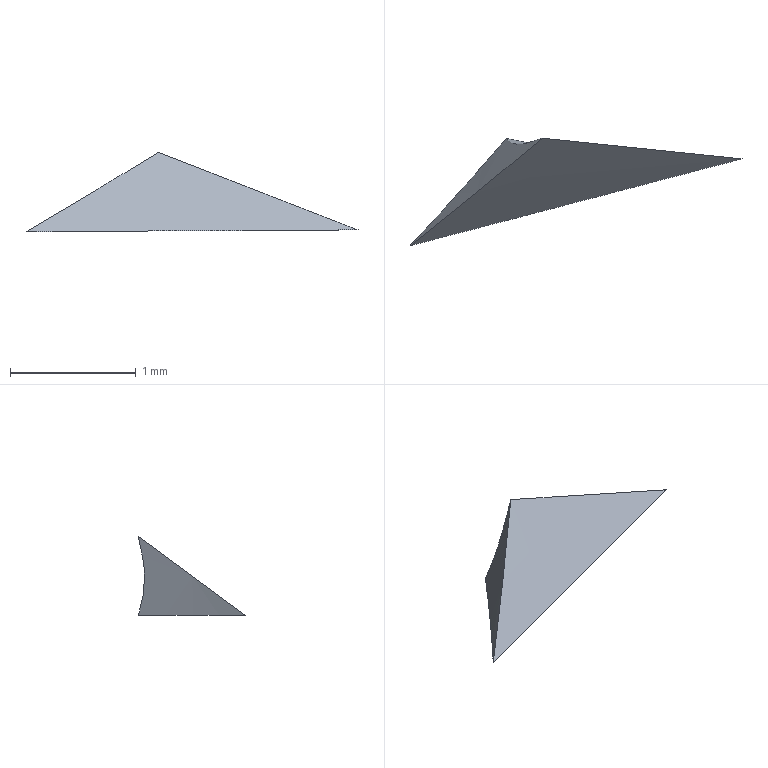Part | STEP file | solid 157 | 1 solid | 5 faces | box 2.637 x 0.8538 x 0.6297 mm | volume 0.1595 mm3 | spline 3 | plane 1 | cylinder 1 | commonest cylinder face diameters 50 x1